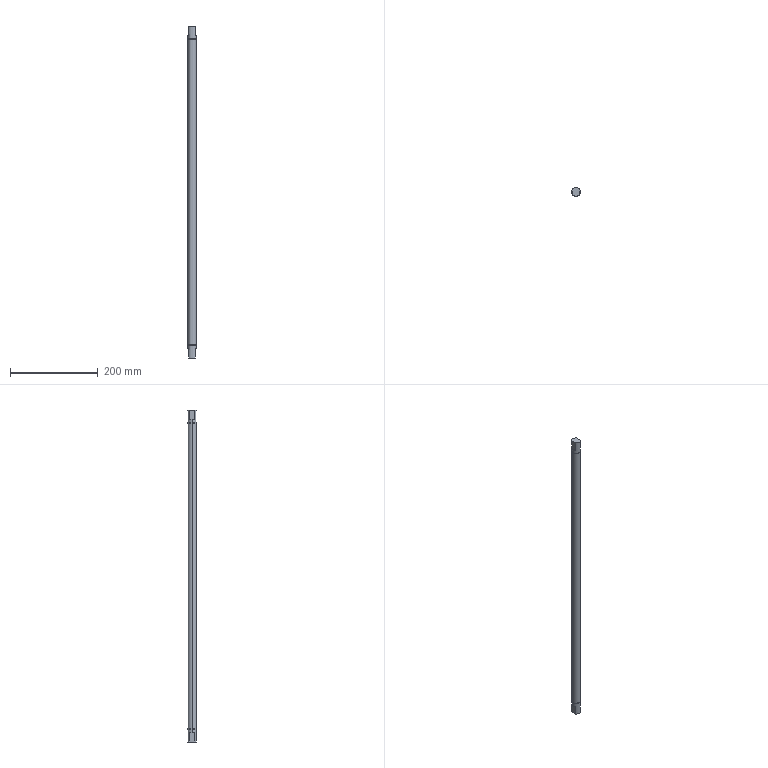Part | SolidWorks | features ICE 2, Extrusion 1, MirrorPattern 1 | 1 solid | 24 faces | box 20 x 20 x 755 mm | volume 235219 mm3 | plane 14 | cylinder 10 | commonest cylinder face diameters 20 x6 19 x4
STEP:
#1=CARTESIAN_POINT('',(7.5,6.614,356.5));
#2=VERTEX_POINT('',#1);
#3=CARTESIAN_POINT('',(10.,0.,356.5));
#4=VERTEX_POINT('',#3);
#5=CARTESIAN_POINT('',(0.,0.,356.5));
#6=DIRECTION('',(0.,0.,-1.));
#7=DIRECTION('',(-1.,0.,0.));
#8=AXIS2_PLACEMENT_3D('',#5,#6,#7);
#9=CIRCLE('',#8,10.);
#10=EDGE_CURVE('',#2,#4,#9,.T.);
#11=ORIENTED_EDGE('',*,*,#10,.T.);
#12=CARTESIAN_POINT('',(10.,0.,348.6));
#13=VERTEX_POINT('',#12);
#14=CARTESIAN_POINT('',(10.,0.,377.5));
#15=DIRECTION('',(0.,0.,-1.));
#16=VECTOR('',#15,1000.);
#17=LINE('',#14,#16);
#18=EDGE_CURVE('',#4,#13,#17,.T.);
#19=ORIENTED_EDGE('',*,*,#18,.T.);
#20=CARTESIAN_POINT('',(-10.,0.,348.6));
#21=VERTEX_POINT('',#20);
#22=CARTESIAN_POINT('',(0.,0.,348.6));
#23=DIRECTION('',(0.,0.,-1.));
#24=DIRECTION('',(-1.,0.,0.));
#25=AXIS2_PLACEMENT_3D('',#22,#23,#24);
#26=CIRCLE('',#25,10.);
#27=EDGE_CURVE('',#21,#13,#26,.T.);
#28=ORIENTED_EDGE('',*,*,#27,.F.);
#29=CARTESIAN_POINT('',(-10.,0.,356.5));
#30=VERTEX_POINT('',#29);
#31=CARTESIAN_POINT('',(-10.,0.,377.5));
#32=DIRECTION('',(0.,0.,-1.));
#33=VECTOR('',#32,1000.);
#34=LINE('',#31,#33);
#35=EDGE_CURVE('',#30,#21,#34,.T.);
#36=ORIENTED_EDGE('',*,*,#35,.F.);
#37=CARTESIAN_POINT('',(-7.5,6.614,356.5));
#38=VERTEX_POINT('',#37);
#39=CARTESIAN_POINT('',(0.,0.,356.5));
#40=DIRECTION('',(0.,0.,-1.));
#41=DIRECTION('',(-1.,0.,0.));
#42=AXIS2_PLACEMENT_3D('',#39,#40,#41);
#43=CIRCLE('',#42,10.);
#44=EDGE_CURVE('',#30,#38,#43,.T.);
#45=ORIENTED_EDGE('',*,*,#44,.T.);
#46=CARTESIAN_POINT('',(-7.5,6.614,377.5));
#47=VERTEX_POINT('',#46);
#48=CARTESIAN_POINT('',(-7.5,6.614,377.5));
#49=DIRECTION('',(0.,0.,1.));
#50=VECTOR('',#49,1000.);
#51=LINE('',#48,#50);
#52=EDGE_CURVE('',#38,#47,#51,.T.);
#53=ORIENTED_EDGE('',*,*,#52,.T.);
#54=CARTESIAN_POINT('',(7.5,6.614,377.5));
#55=VERTEX_POINT('',#54);
#56=CARTESIAN_POINT('',(0.,0.,377.5));
#57=DIRECTION('',(0.,0.,1.));
#58=DIRECTION('',(1.,0.,0.));
#59=AXIS2_PLACEMENT_3D('',#56,#57,#58);
#60=CIRCLE('',#59,10.);
#61=EDGE_CURVE('',#55,#47,#60,.T.);
#62=ORIENTED_EDGE('',*,*,#61,.F.);
#63=CARTESIAN_POINT('',(7.5,6.614,377.5));
#64=DIRECTION('',(0.,0.,-1.));
#65=VECTOR('',#64,1000.);
#66=LINE('',#63,#65);
#67=EDGE_CURVE('',#55,#2,#66,.T.);
#68=ORIENTED_EDGE('',*,*,#67,.T.);
#69=EDGE_LOOP('',(#11,#19,#28,#36,#45,#53,#62,#68));
#70=FACE_OUTER_BOUND('',#69,.T.);
#71=CARTESIAN_POINT('',(0.,0.,377.5));
#72=DIRECTION('',(0.,0.,-1.));
#73=DIRECTION('',(-1.,0.,0.));
#74=AXIS2_PLACEMENT_3D('',#71,#72,#73);
#75=CYLINDRICAL_SURFACE('',#74,10.);
#76=ADVANCED_FACE('',(#70),#75,.T.);
#77=CARTESIAN_POINT('',(-9.5,0.,348.6));
#78=VERTEX_POINT('',#77);
#79=CARTESIAN_POINT('',(9.5,0.,348.6));
#80=VERTEX_POINT('',#79);
#81=CARTESIAN_POINT('',(0.,0.,348.6));
#82=DIRECTION('',(0.,0.,-1.));
#83=DIRECTION('',(-1.,0.,0.));
#84=AXIS2_PLACEMENT_3D('',#81,#82,#83);
#85=CIRCLE('',#84,9.5);
#86=EDGE_CURVE('',#78,#80,#85,.T.);
#87=ORIENTED_EDGE('',*,*,#86,.T.);
#88=CARTESIAN_POINT('',(9.5,0.,347.5));
#89=VERTEX_POINT('',#88);
#90=CARTESIAN_POINT('',(9.5,0.,348.6));
#91=DIRECTION('',(0.,0.,-1.));
#92=VECTOR('',#91,1000.);
#93=LINE('',#90,#92);
#94=EDGE_CURVE('',#80,#89,#93,.T.);
#95=ORIENTED_EDGE('',*,*,#94,.T.);
#96=CARTESIAN_POINT('',(-9.5,0.,347.5));
#97=VERTEX_POINT('',#96);
#98=CARTESIAN_POINT('',(0.,0.,347.5));
#99=DIRECTION('',(0.,0.,-1.));
#100=DIRECTION('',(-1.,0.,0.));
#101=AXIS2_PLACEMENT_3D('',#98,#99,#100);
#102=CIRCLE('',#101,9.5);
#103=EDGE_CURVE('',#97,#89,#102,.T.);
#104=ORIENTED_EDGE('',*,*,#103,.F.);
#105=CARTESIAN_POINT('',(-9.5,0.,348.6));
#106=DIRECTION('',(0.,0.,-1.));
#107=VECTOR('',#106,1000.);
#108=LINE('',#105,#107);
#109=EDGE_CURVE('',#78,#97,#108,.T.);
#110=ORIENTED_EDGE('',*,*,#109,.F.);
#111=EDGE_LOOP('',(#87,#95,#104,#110));
#112=FACE_OUTER_BOUND('',#111,.T.);
#113=CARTESIAN_POINT('',(0.,0.,348.6));
#114=DIRECTION('',(0.,0.,-1.));
#115=DIRECTION('',(-1.,0.,0.));
#116=AXIS2_PLACEMENT_3D('',#113,#114,#115);
#117=CYLINDRICAL_SURFACE('',#116,9.5);
#118=ADVANCED_FACE('',(#112),#117,.T.);
#119=CARTESIAN_POINT('',(-9.5,0.,-348.6));
#120=VERTEX_POINT('',#119);
#121=CARTESIAN_POINT('',(9.5,0.,-348.6));
#122=VERTEX_POINT('',#121);
#123=CARTESIAN_POINT('',(0.,0.,-348.6));
#124=DIRECTION('',(0.,0.,-1.));
#125=DIRECTION('',(-1.,0.,0.));
#126=AXIS2_PLACEMENT_3D('',#123,#124,#125);
#127=CIRCLE('',#126,9.5);
#128=EDGE_CURVE('',#120,#122,#127,.T.);
#129=ORIENTED_EDGE('',*,*,#128,.F.);
#130=CARTESIAN_POINT('',(-9.5,0.,-347.5));
#131=VERTEX_POINT('',#130);
#132=CARTESIAN_POINT('',(-9.5,0.,-348.6));
#133=DIRECTION('',(0.,0.,1.));
#134=VECTOR('',#133,1000.);
#135=LINE('',#132,#134);
#136=EDGE_CURVE('',#120,#131,#135,.T.);
#137=ORIENTED_EDGE('',*,*,#136,.T.);
#138=CARTESIAN_POINT('',(9.5,0.,-347.5));
#139=VERTEX_POINT('',#138);
#140=CARTESIAN_POINT('',(0.,0.,-347.5));
#141=DIRECTION('',(0.,0.,-1.));
#142=DIRECTION('',(-1.,0.,0.));
#143=AXIS2_PLACEMENT_3D('',#140,#141,#142);
#144=CIRCLE('',#143,9.5);
#145=EDGE_CURVE('',#131,#139,#144,.T.);
#146=ORIENTED_EDGE('',*,*,#145,.T.);
#147=CARTESIAN_POINT('',(9.5,0.,-348.6));
#148=DIRECTION('',(0.,0.,1.));
#149=VECTOR('',#148,1000.);
#150=LINE('',#147,#149);
#151=EDGE_CURVE('',#122,#139,#150,.T.);
#152=ORIENTED_EDGE('',*,*,#151,.F.);
#153=EDGE_LOOP('',(#129,#137,#146,#152));
#154=FACE_OUTER_BOUND('',#153,.T.);
#155=CARTESIAN_POINT('',(0.,0.,-348.6));
#156=DIRECTION('',(0.,0.,1.));
#157=DIRECTION('',(1.,0.,0.));
#158=AXIS2_PLACEMENT_3D('',#155,#156,#157);
#159=CYLINDRICAL_SURFACE('',#158,9.5);
#160=ADVANCED_FACE('',(#154),#159,.T.);
#161=CARTESIAN_POINT('',(-10.,0.,-348.6));
#162=VERTEX_POINT('',#161);
#163=CARTESIAN_POINT('',(10.,0.,-348.6));
#164=VERTEX_POINT('',#163);
#165=CARTESIAN_POINT('',(0.,0.,-348.6));
#166=DIRECTION('',(0.,0.,-1.));
#167=DIRECTION('',(-1.,0.,0.));
#168=AXIS2_PLACEMENT_3D('',#165,#166,#167);
#169=CIRCLE('',#168,10.);
#170=EDGE_CURVE('',#162,#164,#169,.T.);
#171=ORIENTED_EDGE('',*,*,#170,.T.);
#172=CARTESIAN_POINT('',(10.,0.,-356.5));
#173=VERTEX_POINT('',#172);
#174=CARTESIAN_POINT('',(10.,0.,377.5));
#175=DIRECTION('',(0.,0.,-1.));
#176=VECTOR('',#175,1000.);
#177=LINE('',#174,#176);
#178=EDGE_CURVE('',#164,#173,#177,.T.);
#179=ORIENTED_EDGE('',*,*,#178,.T.);
#180=CARTESIAN_POINT('',(7.5,6.614,-356.5));
#181=VERTEX_POINT('',#180);
#182=CARTESIAN_POINT('',(0.,0.,-356.5));
#183=DIRECTION('',(0.,0.,1.));
#184=DIRECTION('',(1.,0.,0.));
#185=AXIS2_PLACEMENT_3D('',#182,#183,#184);
#186=CIRCLE('',#185,10.);
#187=EDGE_CURVE('',#173,#181,#186,.T.);
#188=ORIENTED_EDGE('',*,*,#187,.T.);
#189=CARTESIAN_POINT('',(7.5,6.614,-377.5));
#190=VERTEX_POINT('',#189);
#191=CARTESIAN_POINT('',(7.5,6.614,377.5));
#192=DIRECTION('',(0.,0.,-1.));
#193=VECTOR('',#192,1000.);
#194=LINE('',#191,#193);
#195=EDGE_CURVE('',#181,#190,#194,.T.);
#196=ORIENTED_EDGE('',*,*,#195,.T.);
#197=CARTESIAN_POINT('',(-7.5,6.614,-377.5));
#198=VERTEX_POINT('',#197);
#199=CARTESIAN_POINT('',(0.,0.,-377.5));
#200=DIRECTION('',(0.,0.,1.));
#201=DIRECTION('',(1.,0.,0.));
#202=AXIS2_PLACEMENT_3D('',#199,#200,#201);
#203=CIRCLE('',#202,10.);
#204=EDGE_CURVE('',#190,#198,#203,.T.);
#205=ORIENTED_EDGE('',*,*,#204,.T.);
#206=CARTESIAN_POINT('',(-7.5,6.614,-356.5));
#207=VERTEX_POINT('',#206);
#208=CARTESIAN_POINT('',(-7.5,6.614,377.5));
#209=DIRECTION('',(0.,0.,1.));
#210=VECTOR('',#209,1000.);
#211=LINE('',#208,#210);
#212=EDGE_CURVE('',#198,#207,#211,.T.);
#213=ORIENTED_EDGE('',*,*,#212,.T.);
#214=CARTESIAN_POINT('',(-10.,0.,-356.5));
#215=VERTEX_POINT('',#214);
#216=CARTESIAN_POINT('',(0.,0.,-356.5));
#217=DIRECTION('',(0.,0.,1.));
#218=DIRECTION('',(1.,0.,0.));
#219=AXIS2_PLACEMENT_3D('',#216,#217,#218);
#220=CIRCLE('',#219,10.);
#221=EDGE_CURVE('',#207,#215,#220,.T.);
#222=ORIENTED_EDGE('',*,*,#221,.T.);
#223=CARTESIAN_POINT('',(-10.,0.,377.5));
#224=DIRECTION('',(0.,0.,-1.));
#225=VECTOR('',#224,1000.);
#226=LINE('',#223,#225);
#227=EDGE_CURVE('',#162,#215,#226,.T.);
#228=ORIENTED_EDGE('',*,*,#227,.F.);
#229=EDGE_LOOP('',(#171,#179,#188,#196,#205,#213,#222,#228));
#230=FACE_OUTER_BOUND('',#229,.T.);
#231=CARTESIAN_POINT('',(0.,0.,377.5));
#232=DIRECTION('',(0.,0.,-1.));
#233=DIRECTION('',(-1.,0.,0.));
#234=AXIS2_PLACEMENT_3D('',#231,#232,#233);
#235=CYLINDRICAL_SURFACE('',#234,10.);
#236=ADVANCED_FACE('',(#230),#235,.T.);
#237=CARTESIAN_POINT('',(-10.,0.,347.5));
#238=VERTEX_POINT('',#237);
#239=CARTESIAN_POINT('',(10.,0.,347.5));
#240=VERTEX_POINT('',#239);
#241=CARTESIAN_POINT('',(0.,0.,347.5));
#242=DIRECTION('',(0.,0.,-1.));
#243=DIRECTION('',(-1.,0.,0.));
#244=AXIS2_PLACEMENT_3D('',#241,#242,#243);
#245=CIRCLE('',#244,10.);
#246=EDGE_CURVE('',#238,#240,#245,.T.);
#247=ORIENTED_EDGE('',*,*,#246,.T.);
#248=CARTESIAN_POINT('',(10.,0.,-347.5));
#249=VERTEX_POINT('',#248);
#250=CARTESIAN_POINT('',(10.,0.,377.5));
#251=DIRECTION('',(0.,0.,-1.));
#252=VECTOR('',#251,1000.);
#253=LINE('',#250,#252);
#254=EDGE_CURVE('',#240,#249,#253,.T.);
#255=ORIENTED_EDGE('',*,*,#254,.T.);
#256=CARTESIAN_POINT('',(-10.,0.,-347.5));
#257=VERTEX_POINT('',#256);
#258=CARTESIAN_POINT('',(0.,0.,-347.5));
#259=DIRECTION('',(0.,0.,-1.));
#260=DIRECTION('',(-1.,0.,0.));
#261=AXIS2_PLACEMENT_3D('',#258,#259,#260);
#262=CIRCLE('',#261,10.);
#263=EDGE_CURVE('',#257,#249,#262,.T.);
#264=ORIENTED_EDGE('',*,*,#263,.F.);
#265=CARTESIAN_POINT('',(-10.,0.,377.5));
#266=DIRECTION('',(0.,0.,-1.));
#267=VECTOR('',#266,1000.);
#268=LINE('',#265,#267);
#269=EDGE_CURVE('',#238,#257,#268,.T.);
#270=ORIENTED_EDGE('',*,*,#269,.F.);
#271=EDGE_LOOP('',(#247,#255,#264,#270));
#272=FACE_OUTER_BOUND('',#271,.T.);
#273=CARTESIAN_POINT('',(0.,0.,377.5));
#274=DIRECTION('',(0.,0.,-1.));
#275=DIRECTION('',(-1.,0.,0.));
#276=AXIS2_PLACEMENT_3D('',#273,#274,#275);
#277=CYLINDRICAL_SURFACE('',#276,10.);
#278=ADVANCED_FACE('',(#272),#277,.T.);
#279=ORIENTED_EDGE('',*,*,#254,.F.);
#280=CARTESIAN_POINT('',(0.,0.,347.5));
#281=DIRECTION('',(0.,0.,-1.));
#282=DIRECTION('',(-1.,0.,0.));
#283=AXIS2_PLACEMENT_3D('',#280,#281,#282);
#284=CIRCLE('',#283,10.);
#285=EDGE_CURVE('',#240,#238,#284,.T.);
#286=ORIENTED_EDGE('',*,*,#285,.T.);
#287=ORIENTED_EDGE('',*,*,#269,.T.);
#288=CARTESIAN_POINT('',(0.,0.,-347.5));
#289=DIRECTION('',(0.,0.,-1.));
#290=DIRECTION('',(-1.,0.,0.));
#291=AXIS2_PLACEMENT_3D('',#288,#289,#290);
#292=CIRCLE('',#291,10.);
#293=EDGE_CURVE('',#249,#257,#292,.T.);
#294=ORIENTED_EDGE('',*,*,#293,.F.);
#295=EDGE_LOOP('',(#279,#286,#287,#294));
#296=FACE_OUTER_BOUND('',#295,.T.);
#297=CARTESIAN_POINT('',(0.,0.,377.5));
#298=DIRECTION('',(0.,0.,-1.));
#299=DIRECTION('',(-1.,0.,0.));
#300=AXIS2_PLACEMENT_3D('',#297,#298,#299);
#301=CYLINDRICAL_SURFACE('',#300,10.);
#302=ADVANCED_FACE('',(#296),#301,.T.);
#303=ORIENTED_EDGE('',*,*,#178,.F.);
#304=CARTESIAN_POINT('',(0.,0.,-348.6));
#305=DIRECTION('',(0.,0.,-1.));
#306=DIRECTION('',(-1.,0.,0.));
#307=AXIS2_PLACEMENT_3D('',#304,#305,#306);
#308=CIRCLE('',#307,10.);
#309=EDGE_CURVE('',#164,#162,#308,.T.);
#310=ORIENTED_EDGE('',*,*,#309,.T.);
#311=ORIENTED_EDGE('',*,*,#227,.T.);
#312=CARTESIAN_POINT('',(-7.5,-6.614,-356.5));
#313=VERTEX_POINT('',#312);
#314=CARTESIAN_POINT('',(0.,0.,-356.5));
#315=DIRECTION('',(0.,0.,1.));
#316=DIRECTION('',(1.,0.,0.));
#317=AXIS2_PLACEMENT_3D('',#314,#315,#316);
#318=CIRCLE('',#317,10.);
#319=EDGE_CURVE('',#215,#313,#318,.T.);
#320=ORIENTED_EDGE('',*,*,#319,.T.);
#321=CARTESIAN_POINT('',(-7.5,-6.614,-377.5));
#322=VERTEX_POINT('',#321);
#323=CARTESIAN_POINT('',(-7.5,-6.614,377.5));
#324=DIRECTION('',(0.,0.,-1.));
#325=VECTOR('',#324,1000.);
#326=LINE('',#323,#325);
#327=EDGE_CURVE('',#313,#322,#326,.T.);
#328=ORIENTED_EDGE('',*,*,#327,.T.);
#329=CARTESIAN_POINT('',(7.5,-6.614,-377.5));
#330=VERTEX_POINT('',#329);
#331=CARTESIAN_POINT('',(0.,0.,-377.5));
#332=DIRECTION('',(0.,0.,1.));
#333=DIRECTION('',(1.,0.,0.));
#334=AXIS2_PLACEMENT_3D('',#331,#332,#333);
#335=CIRCLE('',#334,10.);
#336=EDGE_CURVE('',#322,#330,#335,.T.);
#337=ORIENTED_EDGE('',*,*,#336,.T.);
#338=CARTESIAN_POINT('',(7.5,-6.614,-356.5));
#339=VERTEX_POINT('',#338);
#340=CARTESIAN_POINT('',(7.5,-6.614,377.5));
#341=DIRECTION('',(0.,0.,1.));
#342=VECTOR('',#341,1000.);
#343=LINE('',#340,#342);
#344=EDGE_CURVE('',#330,#339,#343,.T.);
#345=ORIENTED_EDGE('',*,*,#344,.T.);
#346=CARTESIAN_POINT('',(0.,0.,-356.5));
#347=DIRECTION('',(0.,0.,1.));
#348=DIRECTION('',(1.,0.,0.));
#349=AXIS2_PLACEMENT_3D('',#346,#347,#348);
#350=CIRCLE('',#349,10.);
#351=EDGE_CURVE('',#339,#173,#350,.T.);
#352=ORIENTED_EDGE('',*,*,#351,.T.);
#353=EDGE_LOOP('',(#303,#310,#311,#320,#328,#337,#345,#352));
#354=FACE_OUTER_BOUND('',#353,.T.);
#355=CARTESIAN_POINT('',(0.,0.,377.5));
#356=DIRECTION('',(0.,0.,-1.));
#357=DIRECTION('',(-1.,0.,0.));
#358=AXIS2_PLACEMENT_3D('',#355,#356,#357);
#359=CYLINDRICAL_SURFACE('',#358,10.);
#360=ADVANCED_FACE('',(#354),#359,.T.);
#361=ORIENTED_EDGE('',*,*,#204,.F.);
#362=CARTESIAN_POINT('',(7.5,0.,-377.5));
#363=DIRECTION('',(0.,-1.,0.));
#364=VECTOR('',#363,1000.);
#365=LINE('',#362,#364);
#366=EDGE_CURVE('',#190,#330,#365,.T.);
#367=ORIENTED_EDGE('',*,*,#366,.T.);
#368=ORIENTED_EDGE('',*,*,#336,.F.);
#369=CARTESIAN_POINT('',(-7.5,0.,-377.5));
#370=DIRECTION('',(0.,1.,0.));
#371=VECTOR('',#370,1000.);
#372=LINE('',#369,#371);
#373=EDGE_CURVE('',#322,#198,#372,.T.);
#374=ORIENTED_EDGE('',*,*,#373,.T.);
#375=EDGE_LOOP('',(#361,#367,#368,#374));
#376=FACE_OUTER_BOUND('',#375,.T.);
#377=CARTESIAN_POINT('',(0.,0.,-377.5));
#378=DIRECTION('',(0.,0.,1.));
#379=DIRECTION('',(1.,0.,0.));
#380=AXIS2_PLACEMENT_3D('',#377,#378,#379);
#381=PLANE('',#380);
#382=ADVANCED_FACE('',(#376),#381,.F.);
#383=CARTESIAN_POINT('',(-7.5,-25.,-356.5));
#384=DIRECTION('',(0.,1.,0.));
#385=VECTOR('',#384,1000.);
#386=LINE('',#383,#385);
#387=EDGE_CURVE('',#313,#207,#386,.T.);
#388=ORIENTED_EDGE('',*,*,#387,.F.);
#389=ORIENTED_EDGE('',*,*,#319,.F.);
#390=ORIENTED_EDGE('',*,*,#221,.F.);
#391=EDGE_LOOP('',(#388,#389,#390));
#392=FACE_OUTER_BOUND('',#391,.T.);
#393=CARTESIAN_POINT('',(-28.404,-25.,-356.5));
#394=DIRECTION('',(0.,0.,1.));
#395=DIRECTION('',(1.,0.,0.));
#396=AXIS2_PLACEMENT_3D('',#393,#394,#395);
#397=PLANE('',#396);
#398=ADVANCED_FACE('',(#392),#397,.F.);
#399=ORIENTED_EDGE('',*,*,#387,.T.);
#400=ORIENTED_EDGE('',*,*,#212,.F.);
#401=ORIENTED_EDGE('',*,*,#373,.F.);
#402=ORIENTED_EDGE('',*,*,#327,.F.);
#403=EDGE_LOOP('',(#399,#400,#401,#402));
#404=FACE_OUTER_BOUND('',#403,.T.);
#405=CARTESIAN_POINT('',(-7.5,-25.,-377.5));
#406=DIRECTION('',(1.,0.,0.));
#407=DIRECTION('',(0.,0.,-1.));
#408=AXIS2_PLACEMENT_3D('',#405,#406,#407);
#409=PLANE('',#408);
#410=ADVANCED_FACE('',(#404),#409,.F.);
#411=CARTESIAN_POINT('',(7.5,-25.,-356.5));
#412=DIRECTION('',(0.,1.,0.));
#413=VECTOR('',#412,1000.);
#414=LINE('',#411,#413);
#415=EDGE_CURVE('',#339,#181,#414,.T.);
#416=ORIENTED_EDGE('',*,*,#415,.T.);
#417=ORIENTED_EDGE('',*,*,#187,.F.);
#418=ORIENTED_EDGE('',*,*,#351,.F.);
#419=EDGE_LOOP('',(#416,#417,#418));
#420=FACE_OUTER_BOUND('',#419,.T.);
#421=CARTESIAN_POINT('',(28.404,-25.,-356.5));
#422=DIRECTION('',(0.,0.,1.));
#423=DIRECTION('',(1.,0.,0.));
#424=AXIS2_PLACEMENT_3D('',#421,#422,#423);
#425=PLANE('',#424);
#426=ADVANCED_FACE('',(#420),#425,.F.);
#427=ORIENTED_EDGE('',*,*,#415,.F.);
#428=ORIENTED_EDGE('',*,*,#344,.F.);
#429=ORIENTED_EDGE('',*,*,#366,.F.);
#430=ORIENTED_EDGE('',*,*,#195,.F.);
#431=EDGE_LOOP('',(#427,#428,#429,#430));
#432=FACE_OUTER_BOUND('',#431,.T.);
#433=CARTESIAN_POINT('',(7.5,-25.,-377.5));
#434=DIRECTION('',(-1.,0.,0.));
#435=DIRECTION('',(0.,0.,1.));
#436=AXIS2_PLACEMENT_3D('',#433,#434,#435);
#437=PLANE('',#436);
#438=ADVANCED_FACE('',(#432),#437,.F.);
#439=ORIENTED_EDGE('',*,*,#170,.F.);
#440=ORIENTED_EDGE('',*,*,#309,.F.);
#441=EDGE_LOOP('',(#439,#440));
#442=FACE_OUTER_BOUND('',#441,.T.);
#443=CARTESIAN_POINT('',(0.,0.,-348.6));
#444=DIRECTION('',(0.,0.,-1.));
#445=DIRECTION('',(-1.,0.,0.));
#446=AXIS2_PLACEMENT_3D('',#443,#444,#445);
#447=CIRCLE('',#446,9.5);
#448=EDGE_CURVE('',#122,#120,#447,.T.);
#449=ORIENTED_EDGE('',*,*,#448,.T.);
#450=ORIENTED_EDGE('',*,*,#128,.T.);
#451=EDGE_LOOP('',(#449,#450));
#452=FACE_BOUND('',#451,.T.);
#453=CARTESIAN_POINT('',(0.,0.,-348.6));
#454=DIRECTION('',(0.,0.,-1.));
#455=DIRECTION('',(-1.,0.,0.));
#456=AXIS2_PLACEMENT_3D('',#453,#454,#455);
#457=PLANE('',#456);
#458=ADVANCED_FACE('',(#442,#452),#457,.F.);
#459=ORIENTED_EDGE('',*,*,#263,.T.);
#460=ORIENTED_EDGE('',*,*,#293,.T.);
#461=EDGE_LOOP('',(#459,#460));
#462=FACE_OUTER_BOUND('',#461,.T.);
#463=CARTESIAN_POINT('',(0.,0.,-347.5));
#464=DIRECTION('',(0.,0.,-1.));
#465=DIRECTION('',(-1.,0.,0.));
#466=AXIS2_PLACEMENT_3D('',#463,#464,#465);
#467=CIRCLE('',#466,9.5);
#468=EDGE_CURVE('',#139,#131,#467,.T.);
#469=ORIENTED_EDGE('',*,*,#468,.F.);
#470=ORIENTED_EDGE('',*,*,#145,.F.);
#471=EDGE_LOOP('',(#469,#470));
#472=FACE_BOUND('',#471,.T.);
#473=CARTESIAN_POINT('',(0.,0.,-347.5));
#474=DIRECTION('',(0.,0.,-1.));
#475=DIRECTION('',(-1.,0.,0.));
#476=AXIS2_PLACEMENT_3D('',#473,#474,#475);
#477=PLANE('',#476);
#478=ADVANCED_FACE('',(#462,#472),#477,.T.);
#479=ORIENTED_EDGE('',*,*,#136,.F.);
#480=ORIENTED_EDGE('',*,*,#448,.F.);
#481=ORIENTED_EDGE('',*,*,#151,.T.);
#482=ORIENTED_EDGE('',*,*,#468,.T.);
#483=EDGE_LOOP('',(#479,#480,#481,#482));
#484=FACE_OUTER_BOUND('',#483,.T.);
#485=CARTESIAN_POINT('',(0.,0.,-348.6));
#486=DIRECTION('',(0.,0.,1.));
#487=DIRECTION('',(1.,0.,0.));
#488=AXIS2_PLACEMENT_3D('',#485,#486,#487);
#489=CYLINDRICAL_SURFACE('',#488,9.5);
#490=ADVANCED_FACE('',(#484),#489,.T.);
#491=ORIENTED_EDGE('',*,*,#86,.F.);
#492=CARTESIAN_POINT('',(0.,0.,348.6));
#493=DIRECTION('',(0.,0.,-1.));
#494=DIRECTION('',(-1.,0.,0.));
#495=AXIS2_PLACEMENT_3D('',#492,#493,#494);
#496=CIRCLE('',#495,9.5);
#497=EDGE_CURVE('',#80,#78,#496,.T.);
#498=ORIENTED_EDGE('',*,*,#497,.F.);
#499=EDGE_LOOP('',(#491,#498));
#500=FACE_BOUND('',#499,.T.);
#501=ORIENTED_EDGE('',*,*,#27,.T.);
#502=CARTESIAN_POINT('',(0.,0.,348.6));
#503=DIRECTION('',(0.,0.,-1.));
#504=DIRECTION('',(-1.,0.,0.));
#505=AXIS2_PLACEMENT_3D('',#502,#503,#504);
#506=CIRCLE('',#505,10.);
#507=EDGE_CURVE('',#13,#21,#506,.T.);
#508=ORIENTED_EDGE('',*,*,#507,.T.);
#509=EDGE_LOOP('',(#501,#508));
#510=FACE_OUTER_BOUND('',#509,.T.);
#511=CARTESIAN_POINT('',(0.,0.,348.6));
#512=DIRECTION('',(0.,0.,1.));
#513=DIRECTION('',(-1.,0.,0.));
#514=AXIS2_PLACEMENT_3D('',#511,#512,#513);
#515=PLANE('',#514);
#516=ADVANCED_FACE('',(#500,#510),#515,.F.);
#517=ORIENTED_EDGE('',*,*,#103,.T.);
#518=CARTESIAN_POINT('',(0.,0.,347.5));
#519=DIRECTION('',(0.,0.,-1.));
#520=DIRECTION('',(-1.,0.,0.));
#521=AXIS2_PLACEMENT_3D('',#518,#519,#520);
#522=CIRCLE('',#521,9.5);
#523=EDGE_CURVE('',#89,#97,#522,.T.);
#524=ORIENTED_EDGE('',*,*,#523,.T.);
#525=EDGE_LOOP('',(#517,#524));
#526=FACE_BOUND('',#525,.T.);
#527=ORIENTED_EDGE('',*,*,#246,.F.);
#528=ORIENTED_EDGE('',*,*,#285,.F.);
#529=EDGE_LOOP('',(#527,#528));
#530=FACE_OUTER_BOUND('',#529,.T.);
#531=CARTESIAN_POINT('',(0.,0.,347.5));
#532=DIRECTION('',(0.,0.,1.));
#533=DIRECTION('',(-1.,0.,0.));
#534=AXIS2_PLACEMENT_3D('',#531,#532,#533);
#535=PLANE('',#534);
#536=ADVANCED_FACE('',(#526,#530),#535,.T.);
#537=ORIENTED_EDGE('',*,*,#94,.F.);
#538=ORIENTED_EDGE('',*,*,#497,.T.);
#539=ORIENTED_EDGE('',*,*,#109,.T.);
#540=ORIENTED_EDGE('',*,*,#523,.F.);
#541=EDGE_LOOP('',(#537,#538,#539,#540));
#542=FACE_OUTER_BOUND('',#541,.T.);
#543=CARTESIAN_POINT('',(0.,0.,348.6));
#544=DIRECTION('',(0.,0.,-1.));
#545=DIRECTION('',(-1.,0.,0.));
#546=AXIS2_PLACEMENT_3D('',#543,#544,#545);
#547=CYLINDRICAL_SURFACE('',#546,9.5);
#548=ADVANCED_FACE('',(#542),#547,.T.);
#549=CARTESIAN_POINT('',(7.5,-6.614,356.5));
#550=VERTEX_POINT('',#549);
#551=CARTESIAN_POINT('',(7.5,-25.,356.5));
#552=DIRECTION('',(0.,1.,0.));
#553=VECTOR('',#552,1000.);
#554=LINE('',#551,#553);
#555=EDGE_CURVE('',#550,#2,#554,.T.);
#556=ORIENTED_EDGE('',*,*,#555,.F.);
#557=CARTESIAN_POINT('',(0.,0.,356.5));
#558=DIRECTION('',(0.,0.,-1.));
#559=DIRECTION('',(-1.,0.,0.));
#560=AXIS2_PLACEMENT_3D('',#557,#558,#559);
#561=CIRCLE('',#560,10.);
#562=EDGE_CURVE('',#4,#550,#561,.T.);
#563=ORIENTED_EDGE('',*,*,#562,.F.);
#564=ORIENTED_EDGE('',*,*,#10,.F.);
#565=EDGE_LOOP('',(#556,#563,#564));
#566=FACE_OUTER_BOUND('',#565,.T.);
#567=CARTESIAN_POINT('',(28.404,-25.,356.5));
#568=DIRECTION('',(0.,0.,-1.));
#569=DIRECTION('',(-1.,0.,0.));
#570=AXIS2_PLACEMENT_3D('',#567,#568,#569);
#571=PLANE('',#570);
#572=ADVANCED_FACE('',(#566),#571,.F.);
#573=CARTESIAN_POINT('',(7.5,-6.614,377.5));
#574=VERTEX_POINT('',#573);
#575=CARTESIAN_POINT('',(7.5,0.,377.5));
#576=DIRECTION('',(0.,-1.,0.));
#577=VECTOR('',#576,1000.);
#578=LINE('',#575,#577);
#579=EDGE_CURVE('',#55,#574,#578,.T.);
#580=ORIENTED_EDGE('',*,*,#579,.T.);
#581=CARTESIAN_POINT('',(7.5,-6.614,377.5));
#582=DIRECTION('',(0.,0.,1.));
#583=VECTOR('',#582,1000.);
#584=LINE('',#581,#583);
#585=EDGE_CURVE('',#550,#574,#584,.T.);
#586=ORIENTED_EDGE('',*,*,#585,.F.);
#587=ORIENTED_EDGE('',*,*,#555,.T.);
#588=ORIENTED_EDGE('',*,*,#67,.F.);
#589=EDGE_LOOP('',(#580,#586,#587,#588));
#590=FACE_OUTER_BOUND('',#589,.T.);
#591=CARTESIAN_POINT('',(7.5,-25.,377.5));
#592=DIRECTION('',(-1.,0.,0.));
#593=DIRECTION('',(0.,0.,1.));
#594=AXIS2_PLACEMENT_3D('',#591,#592,#593);
#595=PLANE('',#594);
#596=ADVANCED_FACE('',(#590),#595,.F.);
#597=CARTESIAN_POINT('',(-7.5,-6.614,356.5));
#598=VERTEX_POINT('',#597);
#599=CARTESIAN_POINT('',(-7.5,-25.,356.5));
#600=DIRECTION('',(0.,1.,0.));
#601=VECTOR('',#600,1000.);
#602=LINE('',#599,#601);
#603=EDGE_CURVE('',#598,#38,#602,.T.);
#604=ORIENTED_EDGE('',*,*,#603,.T.);
#605=ORIENTED_EDGE('',*,*,#44,.F.);
#606=CARTESIAN_POINT('',(0.,0.,356.5));
#607=DIRECTION('',(0.,0.,-1.));
#608=DIRECTION('',(-1.,0.,0.));
#609=AXIS2_PLACEMENT_3D('',#606,#607,#608);
#610=CIRCLE('',#609,10.);
#611=EDGE_CURVE('',#598,#30,#610,.T.);
#612=ORIENTED_EDGE('',*,*,#611,.F.);
#613=EDGE_LOOP('',(#604,#605,#612));
#614=FACE_OUTER_BOUND('',#613,.T.);
#615=CARTESIAN_POINT('',(-28.404,-25.,356.5));
#616=DIRECTION('',(0.,0.,-1.));
#617=DIRECTION('',(-1.,0.,0.));
#618=AXIS2_PLACEMENT_3D('',#615,#616,#617);
#619=PLANE('',#618);
#620=ADVANCED_FACE('',(#614),#619,.F.);
#621=CARTESIAN_POINT('',(-7.5,-6.614,377.5));
#622=VERTEX_POINT('',#621);
#623=CARTESIAN_POINT('',(-7.5,0.,377.5));
#624=DIRECTION('',(0.,1.,0.));
#625=VECTOR('',#624,1000.);
#626=LINE('',#623,#625);
#627=EDGE_CURVE('',#622,#47,#626,.T.);
#628=ORIENTED_EDGE('',*,*,#627,.T.);
#629=ORIENTED_EDGE('',*,*,#52,.F.);
#630=ORIENTED_EDGE('',*,*,#603,.F.);
#631=CARTESIAN_POINT('',(-7.5,-6.614,377.5));
#632=DIRECTION('',(0.,0.,-1.));
#633=VECTOR('',#632,1000.);
#634=LINE('',#631,#633);
#635=EDGE_CURVE('',#622,#598,#634,.T.);
#636=ORIENTED_EDGE('',*,*,#635,.F.);
#637=EDGE_LOOP('',(#628,#629,#630,#636));
#638=FACE_OUTER_BOUND('',#637,.T.);
#639=CARTESIAN_POINT('',(-7.5,-25.,377.5));
#640=DIRECTION('',(1.,0.,0.));
#641=DIRECTION('',(0.,0.,-1.));
#642=AXIS2_PLACEMENT_3D('',#639,#640,#641);
#643=PLANE('',#642);
#644=ADVANCED_FACE('',(#638),#643,.F.);
#645=ORIENTED_EDGE('',*,*,#627,.F.);
#646=CARTESIAN_POINT('',(0.,0.,377.5));
#647=DIRECTION('',(0.,0.,1.));
#648=DIRECTION('',(1.,0.,0.));
#649=AXIS2_PLACEMENT_3D('',#646,#647,#648);
#650=CIRCLE('',#649,10.);
#651=EDGE_CURVE('',#622,#574,#650,.T.);
#652=ORIENTED_EDGE('',*,*,#651,.T.);
#653=ORIENTED_EDGE('',*,*,#579,.F.);
#654=ORIENTED_EDGE('',*,*,#61,.T.);
#655=EDGE_LOOP('',(#645,#652,#653,#654));
#656=FACE_OUTER_BOUND('',#655,.T.);
#657=CARTESIAN_POINT('',(0.,0.,377.5));
#658=DIRECTION('',(0.,0.,1.));
#659=DIRECTION('',(1.,0.,0.));
#660=AXIS2_PLACEMENT_3D('',#657,#658,#659);
#661=PLANE('',#660);
#662=ADVANCED_FACE('',(#656),#661,.T.);
#663=ORIENTED_EDGE('',*,*,#18,.F.);
#664=ORIENTED_EDGE('',*,*,#562,.T.);
#665=ORIENTED_EDGE('',*,*,#585,.T.);
#666=ORIENTED_EDGE('',*,*,#651,.F.);
#667=ORIENTED_EDGE('',*,*,#635,.T.);
#668=ORIENTED_EDGE('',*,*,#611,.T.);
#669=ORIENTED_EDGE('',*,*,#35,.T.);
#670=ORIENTED_EDGE('',*,*,#507,.F.);
#671=EDGE_LOOP('',(#663,#664,#665,#666,#667,#668,#669,#670));
#672=FACE_OUTER_BOUND('',#671,.T.);
#673=CARTESIAN_POINT('',(0.,0.,377.5));
#674=DIRECTION('',(0.,0.,-1.));
#675=DIRECTION('',(-1.,0.,0.));
#676=AXIS2_PLACEMENT_3D('',#673,#674,#675);
#677=CYLINDRICAL_SURFACE('',#676,10.);
#678=ADVANCED_FACE('',(#672),#677,.T.);
#679=CLOSED_SHELL('',(#76,#118,#160,#236,#278,#302,#360,#382,#398,#410,#426,#438,#458,#478,#490,#516,#536,#548,#572,#596,#620,#644,#662,#678));
#680=MANIFOLD_SOLID_BREP('',#679);
#681=CARTESIAN_POINT('',(0.,0.,0.));
#682=DIRECTION('',(0.,0.,1.));
#683=DIRECTION('',(1.,0.,0.));
#684=AXIS2_PLACEMENT_3D('',#681,#682,#683);
#685=(LENGTH_UNIT()NAMED_UNIT(*)SI_UNIT(.MILLI.,.METRE.));
#686=UNCERTAINTY_MEASURE_WITH_UNIT(LENGTH_MEASURE(0.00001),#685,'','');
#687=(NAMED_UNIT(*)PLANE_ANGLE_UNIT()SI_UNIT($,.RADIAN.));
#688=(NAMED_UNIT(*)SI_UNIT($,.STERADIAN.)SOLID_ANGLE_UNIT());
#689=(GEOMETRIC_REPRESENTATION_CONTEXT(3)GLOBAL_UNCERTAINTY_ASSIGNED_CONTEXT((#686))GLOBAL_UNIT_ASSIGNED_CONTEXT((#685,#687,#688))REPRESENTATION_CONTEXT('',''));
#690=ADVANCED_BREP_SHAPE_REPRESENTATION('',(#680,#684),#689);